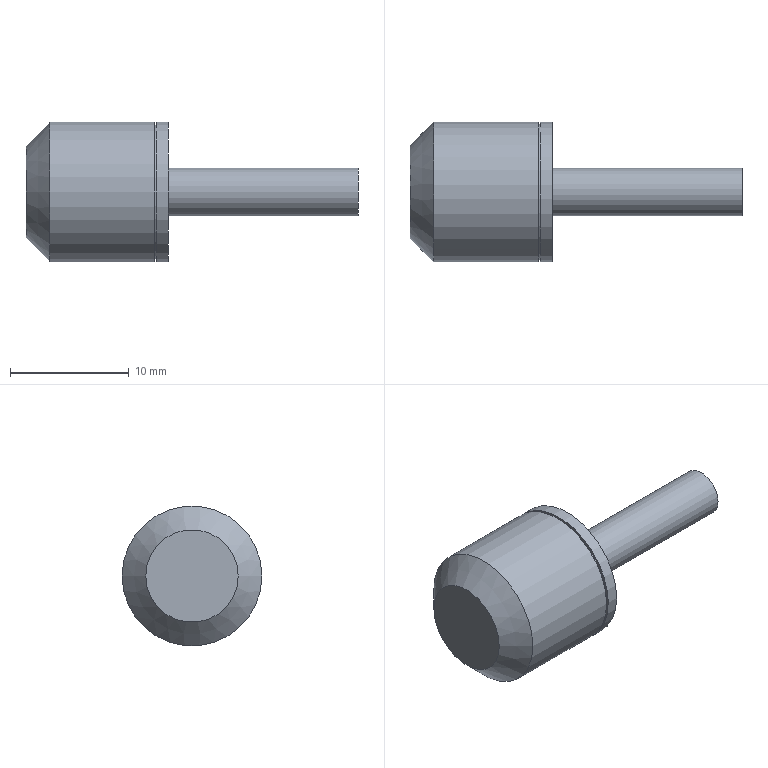Part | NX | features ROD_5003_019_C-AC1412S 2 | 1 solid | 10 faces | box 28 x 11.8 x 11.8 mm | volume 1446 mm3 | plane 5 | cylinder 4 | cone 1 | commonest cylinder face diameters 11.8 x2 4 x1 11.4 x1
STEP:
#1=CARTESIAN_POINT('',(29.1,-142.9,-223.));
#2=VERTEX_POINT('',#1);
#3=CARTESIAN_POINT('',(29.1,-137.,-223.));
#4=DIRECTION('',(-1.,0.,0.));
#5=DIRECTION('',(0.,-1.,0.));
#6=AXIS2_PLACEMENT_3D('',#3,#4,#5);
#7=CIRCLE('',#6,5.9);
#8=EDGE_CURVE('',#2,#2,#7,.T.);
#9=ORIENTED_EDGE('',*,*,#8,.T.);
#10=EDGE_LOOP('',(#9));
#11=FACE_BOUND('',#10,.T.);
#12=CARTESIAN_POINT('',(28.1,-142.9,-223.));
#13=VERTEX_POINT('',#12);
#14=CARTESIAN_POINT('',(28.1,-137.,-223.));
#15=DIRECTION('',(-1.,0.,0.));
#16=DIRECTION('',(0.,-1.,0.));
#17=AXIS2_PLACEMENT_3D('',#14,#15,#16);
#18=CIRCLE('',#17,5.9);
#19=EDGE_CURVE('',#13,#13,#18,.T.);
#20=ORIENTED_EDGE('',*,*,#19,.F.);
#21=EDGE_LOOP('',(#20));
#22=FACE_BOUND('',#21,.T.);
#23=CARTESIAN_POINT('',(18.946,-137.,-223.));
#24=DIRECTION('',(-1.,0.,0.));
#25=DIRECTION('',(0.,-1.,0.));
#26=AXIS2_PLACEMENT_3D('',#23,#24,#25);
#27=CYLINDRICAL_SURFACE('',#26,5.9);
#28=ADVANCED_FACE('',(#11,#22),#27,.T.);
#29=CARTESIAN_POINT('',(29.1,-139.,-223.));
#30=VERTEX_POINT('',#29);
#31=CARTESIAN_POINT('',(29.1,-137.,-223.));
#32=DIRECTION('',(-1.,0.,0.));
#33=DIRECTION('',(0.,-1.,0.));
#34=AXIS2_PLACEMENT_3D('',#31,#32,#33);
#35=CIRCLE('',#34,2.);
#36=EDGE_CURVE('',#30,#30,#35,.T.);
#37=ORIENTED_EDGE('',*,*,#36,.F.);
#38=EDGE_LOOP('',(#37));
#39=FACE_BOUND('',#38,.T.);
#40=CARTESIAN_POINT('',(45.1,-139.,-223.));
#41=VERTEX_POINT('',#40);
#42=CARTESIAN_POINT('',(45.1,-137.,-223.));
#43=DIRECTION('',(-1.,0.,0.));
#44=DIRECTION('',(0.,-1.,0.));
#45=AXIS2_PLACEMENT_3D('',#42,#43,#44);
#46=CIRCLE('',#45,2.);
#47=EDGE_CURVE('',#41,#41,#46,.T.);
#48=ORIENTED_EDGE('',*,*,#47,.T.);
#49=EDGE_LOOP('',(#48));
#50=FACE_BOUND('',#49,.T.);
#51=CARTESIAN_POINT('',(18.946,-137.,-223.));
#52=DIRECTION('',(-1.,0.,0.));
#53=DIRECTION('',(0.,-1.,0.));
#54=AXIS2_PLACEMENT_3D('',#51,#52,#53);
#55=CYLINDRICAL_SURFACE('',#54,2.);
#56=ADVANCED_FACE('',(#39,#50),#55,.T.);
#57=ORIENTED_EDGE('',*,*,#47,.F.);
#58=EDGE_LOOP('',(#57));
#59=FACE_BOUND('',#58,.T.);
#60=CARTESIAN_POINT('',(45.1,-137.,-221.));
#61=DIRECTION('',(-1.,0.,0.));
#62=DIRECTION('',(0.,-1.,0.));
#63=AXIS2_PLACEMENT_3D('',#60,#61,#62);
#64=PLANE('',#63);
#65=ADVANCED_FACE('',(#59),#64,.F.);
#66=ORIENTED_EDGE('',*,*,#8,.F.);
#67=EDGE_LOOP('',(#66));
#68=FACE_BOUND('',#67,.T.);
#69=ORIENTED_EDGE('',*,*,#36,.T.);
#70=EDGE_LOOP('',(#69));
#71=FACE_BOUND('',#70,.T.);
#72=CARTESIAN_POINT('',(29.1,-137.,-217.1));
#73=DIRECTION('',(-1.,0.,0.));
#74=DIRECTION('',(0.,-1.,0.));
#75=AXIS2_PLACEMENT_3D('',#72,#73,#74);
#76=PLANE('',#75);
#77=ADVANCED_FACE('',(#68,#71),#76,.F.);
#78=CARTESIAN_POINT('',(27.9,-142.7,-223.));
#79=VERTEX_POINT('',#78);
#80=CARTESIAN_POINT('',(27.9,-137.,-223.));
#81=DIRECTION('',(-1.,0.,0.));
#82=DIRECTION('',(0.,-1.,0.));
#83=AXIS2_PLACEMENT_3D('',#80,#81,#82);
#84=CIRCLE('',#83,5.7);
#85=EDGE_CURVE('',#79,#79,#84,.T.);
#86=ORIENTED_EDGE('',*,*,#85,.T.);
#87=EDGE_LOOP('',(#86));
#88=FACE_BOUND('',#87,.T.);
#89=CARTESIAN_POINT('',(27.9,-142.9,-223.));
#90=VERTEX_POINT('',#89);
#91=CARTESIAN_POINT('',(27.9,-137.,-223.));
#92=DIRECTION('',(-1.,0.,0.));
#93=DIRECTION('',(0.,-1.,0.));
#94=AXIS2_PLACEMENT_3D('',#91,#92,#93);
#95=CIRCLE('',#94,5.9);
#96=EDGE_CURVE('',#90,#90,#95,.T.);
#97=ORIENTED_EDGE('',*,*,#96,.F.);
#98=EDGE_LOOP('',(#97));
#99=FACE_BOUND('',#98,.T.);
#100=CARTESIAN_POINT('',(27.9,-137.,-217.1));
#101=DIRECTION('',(1.,0.,0.));
#102=DIRECTION('',(0.,1.,0.));
#103=AXIS2_PLACEMENT_3D('',#100,#101,#102);
#104=PLANE('',#103);
#105=ADVANCED_FACE('',(#88,#99),#104,.T.);
#106=CARTESIAN_POINT('',(28.1,-142.7,-223.));
#107=VERTEX_POINT('',#106);
#108=CARTESIAN_POINT('',(28.1,-137.,-223.));
#109=DIRECTION('',(-1.,0.,0.));
#110=DIRECTION('',(0.,-1.,0.));
#111=AXIS2_PLACEMENT_3D('',#108,#109,#110);
#112=CIRCLE('',#111,5.7);
#113=EDGE_CURVE('',#107,#107,#112,.T.);
#114=ORIENTED_EDGE('',*,*,#113,.T.);
#115=EDGE_LOOP('',(#114));
#116=FACE_BOUND('',#115,.T.);
#117=ORIENTED_EDGE('',*,*,#85,.F.);
#118=EDGE_LOOP('',(#117));
#119=FACE_BOUND('',#118,.T.);
#120=CARTESIAN_POINT('',(18.946,-137.,-223.));
#121=DIRECTION('',(-1.,0.,0.));
#122=DIRECTION('',(0.,-1.,0.));
#123=AXIS2_PLACEMENT_3D('',#120,#121,#122);
#124=CYLINDRICAL_SURFACE('',#123,5.7);
#125=ADVANCED_FACE('',(#116,#119),#124,.T.);
#126=ORIENTED_EDGE('',*,*,#19,.T.);
#127=EDGE_LOOP('',(#126));
#128=FACE_BOUND('',#127,.T.);
#129=ORIENTED_EDGE('',*,*,#113,.F.);
#130=EDGE_LOOP('',(#129));
#131=FACE_BOUND('',#130,.T.);
#132=CARTESIAN_POINT('',(28.1,-137.,-217.1));
#133=DIRECTION('',(-1.,0.,0.));
#134=DIRECTION('',(0.,-1.,0.));
#135=AXIS2_PLACEMENT_3D('',#132,#133,#134);
#136=PLANE('',#135);
#137=ADVANCED_FACE('',(#128,#131),#136,.T.);
#138=CARTESIAN_POINT('',(17.1,-140.9,-223.));
#139=VERTEX_POINT('',#138);
#140=CARTESIAN_POINT('',(17.1,-137.,-223.));
#141=DIRECTION('',(-1.,0.,0.));
#142=DIRECTION('',(0.,-1.,0.));
#143=AXIS2_PLACEMENT_3D('',#140,#141,#142);
#144=CIRCLE('',#143,3.9);
#145=EDGE_CURVE('',#139,#139,#144,.T.);
#146=ORIENTED_EDGE('',*,*,#145,.T.);
#147=EDGE_LOOP('',(#146));
#148=FACE_BOUND('',#147,.T.);
#149=CARTESIAN_POINT('',(17.1,-137.,-223.));
#150=DIRECTION('',(1.,0.,0.));
#151=DIRECTION('',(0.,1.,0.));
#152=AXIS2_PLACEMENT_3D('',#149,#150,#151);
#153=PLANE('',#152);
#154=ADVANCED_FACE('',(#148),#153,.F.);
#155=ORIENTED_EDGE('',*,*,#145,.F.);
#156=EDGE_LOOP('',(#155));
#157=FACE_BOUND('',#156,.T.);
#158=CARTESIAN_POINT('',(19.1,-142.9,-223.));
#159=VERTEX_POINT('',#158);
#160=CARTESIAN_POINT('',(19.1,-137.,-223.));
#161=DIRECTION('',(-1.,0.,0.));
#162=DIRECTION('',(0.,-1.,0.));
#163=AXIS2_PLACEMENT_3D('',#160,#161,#162);
#164=CIRCLE('',#163,5.9);
#165=EDGE_CURVE('',#159,#159,#164,.T.);
#166=ORIENTED_EDGE('',*,*,#165,.T.);
#167=EDGE_LOOP('',(#166));
#168=FACE_BOUND('',#167,.T.);
#169=CARTESIAN_POINT('',(19.1,-137.,-223.));
#170=DIRECTION('',(1.,0.,0.));
#171=DIRECTION('',(0.,1.,0.));
#172=AXIS2_PLACEMENT_3D('',#169,#170,#171);
#173=CONICAL_SURFACE('',#172,5.9,0.7854);
#174=ADVANCED_FACE('',(#157,#168),#173,.T.);
#175=ORIENTED_EDGE('',*,*,#165,.F.);
#176=EDGE_LOOP('',(#175));
#177=FACE_BOUND('',#176,.T.);
#178=ORIENTED_EDGE('',*,*,#96,.T.);
#179=EDGE_LOOP('',(#178));
#180=FACE_BOUND('',#179,.T.);
#181=CARTESIAN_POINT('',(18.946,-137.,-223.));
#182=DIRECTION('',(-1.,0.,0.));
#183=DIRECTION('',(0.,-1.,0.));
#184=AXIS2_PLACEMENT_3D('',#181,#182,#183);
#185=CYLINDRICAL_SURFACE('',#184,5.9);
#186=ADVANCED_FACE('',(#177,#180),#185,.T.);
#187=CLOSED_SHELL('',(#28,#56,#65,#77,#105,#125,#137,#154,#174,#186));
#188=MANIFOLD_SOLID_BREP('',#187);
#189=(LENGTH_UNIT()NAMED_UNIT(*)SI_UNIT(.MILLI.,.METRE.));
#190=UNCERTAINTY_MEASURE_WITH_UNIT(LENGTH_MEASURE(0.00001),#189,'','');
#191=(NAMED_UNIT(*)PLANE_ANGLE_UNIT()SI_UNIT($,.RADIAN.));
#192=(NAMED_UNIT(*)SI_UNIT($,.STERADIAN.)SOLID_ANGLE_UNIT());
#193=(GEOMETRIC_REPRESENTATION_CONTEXT(3)GLOBAL_UNCERTAINTY_ASSIGNED_CONTEXT((#190))GLOBAL_UNIT_ASSIGNED_CONTEXT((#189,#191,#192))REPRESENTATION_CONTEXT('',''));
#194=ADVANCED_BREP_SHAPE_REPRESENTATION('',(#188),#193);